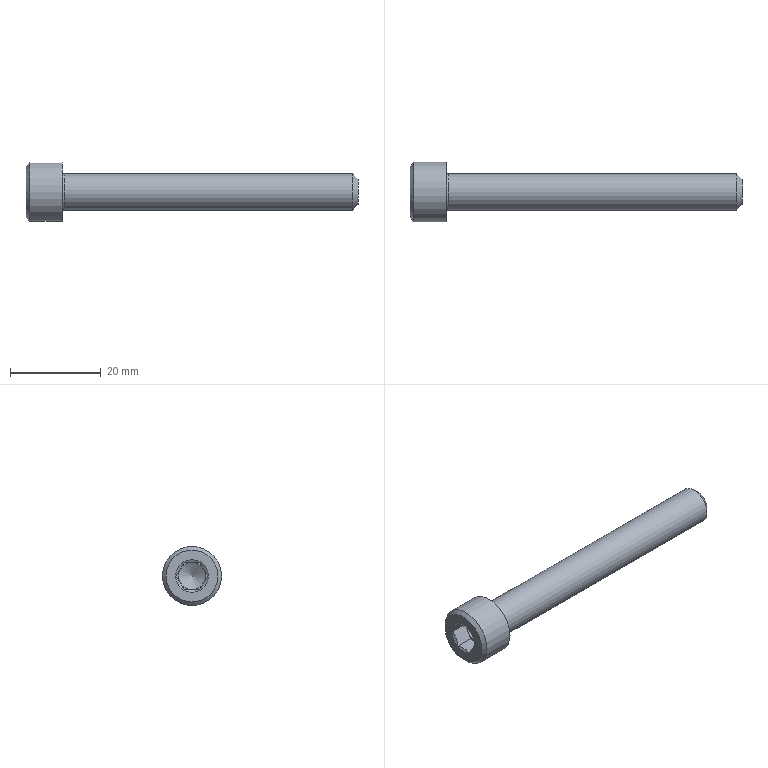Part | STEP file | Винт М8-6gx65 ГОСТ 11738-84 | 1 solid | 23 faces | box 73 x 13 x 13 mm | volume 4129 mm3 | plane 15 | cone 4 | cylinder 3 | torus 1 | commonest cylinder face diameters 6 x1 8 x1 13 x1
STEP:
#1=CARTESIAN_POINT('',(-8.,5.7,0.));
#2=VERTEX_POINT('',#1);
#3=CARTESIAN_POINT('',(-8.,0.,0.));
#4=DIRECTION('',(1.,0.,0.));
#5=DIRECTION('',(0.,1.,0.));
#6=AXIS2_PLACEMENT_3D('',#3,#4,#5);
#7=CIRCLE('',#6,5.7);
#8=EDGE_CURVE('',#2,#2,#7,.T.);
#9=ORIENTED_EDGE('',*,*,#8,.F.);
#10=EDGE_LOOP('',(#9));
#11=FACE_BOUND('',#10,.T.);
#12=CARTESIAN_POINT('',(-8.,3.6,0.));
#13=VERTEX_POINT('',#12);
#14=CARTESIAN_POINT('',(-8.,0.,0.));
#15=DIRECTION('',(1.,0.,0.));
#16=DIRECTION('',(0.,1.,0.));
#17=AXIS2_PLACEMENT_3D('',#14,#15,#16);
#18=CIRCLE('',#17,3.6);
#19=EDGE_CURVE('',#13,#13,#18,.T.);
#20=ORIENTED_EDGE('',*,*,#19,.T.);
#21=EDGE_LOOP('',(#20));
#22=FACE_BOUND('',#21,.T.);
#23=CARTESIAN_POINT('',(-8.,0.,0.));
#24=DIRECTION('',(-1.,0.,0.));
#25=DIRECTION('',(0.,1.,0.));
#26=AXIS2_PLACEMENT_3D('',#23,#24,#25);
#27=PLANE('',#26);
#28=ADVANCED_FACE('',(#11,#22),#27,.T.);
#29=CARTESIAN_POINT('',(-7.922,1.732,-3.));
#30=VERTEX_POINT('',#29);
#31=CARTESIAN_POINT('',(-7.922,-1.732,-3.));
#32=VERTEX_POINT('',#31);
#33=CARTESIAN_POINT('',(-7.922,1.732,-3.));
#34=CARTESIAN_POINT('',(-7.911,1.695,-3.));
#35=CARTESIAN_POINT('',(-7.891,1.625,-3.));
#36=CARTESIAN_POINT('',(-7.871,1.55,-3.));
#37=CARTESIAN_POINT('',(-7.851,1.474,-3.));
#38=CARTESIAN_POINT('',(-7.831,1.391,-3.));
#39=CARTESIAN_POINT('',(-7.803,1.276,-3.));
#40=CARTESIAN_POINT('',(-7.779,1.162,-3.));
#41=CARTESIAN_POINT('',(-7.76,1.068,-3.));
#42=CARTESIAN_POINT('',(-7.736,0.9374,-3.));
#43=CARTESIAN_POINT('',(-7.712,0.7953,-3.));
#44=CARTESIAN_POINT('',(-7.692,0.6398,-3.));
#45=CARTESIAN_POINT('',(-7.676,0.4906,-3.));
#46=CARTESIAN_POINT('',(-7.667,0.3765,-3.));
#47=CARTESIAN_POINT('',(-7.659,0.2523,-3.));
#48=CARTESIAN_POINT('',(-7.655,0.1456,-3.));
#49=CARTESIAN_POINT('',(-7.654,0.04767,-3.));
#50=CARTESIAN_POINT('',(-7.654,-0.05476,-3.));
#51=CARTESIAN_POINT('',(-7.655,-0.115,-3.));
#52=CARTESIAN_POINT('',(-7.658,-0.2282,-3.));
#53=CARTESIAN_POINT('',(-7.665,-0.3516,-3.));
#54=CARTESIAN_POINT('',(-7.676,-0.494,-3.));
#55=CARTESIAN_POINT('',(-7.689,-0.6078,-3.));
#56=CARTESIAN_POINT('',(-7.702,-0.7201,-3.));
#57=CARTESIAN_POINT('',(-7.719,-0.8365,-3.));
#58=CARTESIAN_POINT('',(-7.737,-0.9456,-3.));
#59=CARTESIAN_POINT('',(-7.756,-1.051,-3.));
#60=CARTESIAN_POINT('',(-7.781,-1.173,-3.));
#61=CARTESIAN_POINT('',(-7.808,-1.297,-3.));
#62=CARTESIAN_POINT('',(-7.831,-1.393,-3.));
#63=CARTESIAN_POINT('',(-7.854,-1.486,-3.));
#64=CARTESIAN_POINT('',(-7.882,-1.59,-3.));
#65=CARTESIAN_POINT('',(-7.906,-1.679,-3.));
#66=CARTESIAN_POINT('',(-7.919,-1.723,-3.));
#67=CARTESIAN_POINT('',(-7.922,-1.732,-3.));
#68=B_SPLINE_CURVE_WITH_KNOTS('',3,(#33,#34,#35,#36,#37,#38,#39,#40,#41,#42,#43,#44,#45,#46,#47,#48,#49,#50,#51,#52,#53,#54,#55,#56,#57,#58,#59,#60,#61,#62,#63,#64,#65,#66,#67),.UNSPECIFIED.,.F.,.F.,(4,1,1,1,1,1,1,1,1,1,1,1,1,1,1,1,1,1,1,1,1,1,1,1,1,1,1,1,1,1,1,1,4),(0.,0.03325,0.06137,0.06664,0.1002,0.134,0.1679,0.1994,0.2162,0.2809,0.3222,0.3499,0.4089,0.4198,0.456,0.5,0.5033,0.5434,0.5514,0.5999,0.6487,0.6732,0.6976,0.7453,0.7735,0.7919,0.8363,0.8796,0.9003,0.9208,0.9609,0.9923,1.),.UNSPECIFIED.);
#69=EDGE_CURVE('',#30,#32,#68,.T.);
#70=ORIENTED_EDGE('',*,*,#69,.T.);
#71=CARTESIAN_POINT('',(-4.,-1.732,-3.));
#72=VERTEX_POINT('',#71);
#73=CARTESIAN_POINT('',(-4.,-1.732,-3.));
#74=DIRECTION('',(-1.,0.,0.));
#75=VECTOR('',#74,1.);
#76=LINE('',#73,#75);
#77=EDGE_CURVE('',#72,#32,#76,.T.);
#78=ORIENTED_EDGE('',*,*,#77,.F.);
#79=CARTESIAN_POINT('',(-4.,0.,-3.));
#80=VERTEX_POINT('',#79);
#81=CARTESIAN_POINT('',(-4.,0.,-3.));
#82=DIRECTION('',(0.,-1.,0.));
#83=VECTOR('',#82,1.);
#84=LINE('',#81,#83);
#85=EDGE_CURVE('',#80,#72,#84,.T.);
#86=ORIENTED_EDGE('',*,*,#85,.F.);
#87=CARTESIAN_POINT('',(-4.,1.732,-3.));
#88=VERTEX_POINT('',#87);
#89=CARTESIAN_POINT('',(-4.,1.732,-3.));
#90=DIRECTION('',(0.,-1.,0.));
#91=VECTOR('',#90,1.);
#92=LINE('',#89,#91);
#93=EDGE_CURVE('',#88,#80,#92,.T.);
#94=ORIENTED_EDGE('',*,*,#93,.F.);
#95=CARTESIAN_POINT('',(-4.,1.732,-3.));
#96=DIRECTION('',(-1.,0.,0.));
#97=VECTOR('',#96,1.);
#98=LINE('',#95,#97);
#99=EDGE_CURVE('',#88,#30,#98,.T.);
#100=ORIENTED_EDGE('',*,*,#99,.T.);
#101=EDGE_LOOP('',(#70,#78,#86,#94,#100));
#102=FACE_BOUND('',#101,.T.);
#103=CARTESIAN_POINT('',(-4.,1.732,-3.));
#104=DIRECTION('',(0.,0.,-1.));
#105=DIRECTION('',(0.,-1.,0.));
#106=AXIS2_PLACEMENT_3D('',#103,#104,#105);
#107=PLANE('',#106);
#108=ADVANCED_FACE('',(#102),#107,.F.);
#109=CARTESIAN_POINT('',(-7.922,-3.464,0.));
#110=VERTEX_POINT('',#109);
#111=CARTESIAN_POINT('',(-7.922,-1.732,-3.));
#112=CARTESIAN_POINT('',(-7.911,-1.751,-2.968));
#113=CARTESIAN_POINT('',(-7.89,-1.788,-2.902));
#114=CARTESIAN_POINT('',(-7.859,-1.845,-2.804));
#115=CARTESIAN_POINT('',(-7.831,-1.902,-2.705));
#116=CARTESIAN_POINT('',(-7.803,-1.96,-2.605));
#117=CARTESIAN_POINT('',(-7.775,-2.027,-2.49));
#118=CARTESIAN_POINT('',(-7.741,-2.111,-2.343));
#119=CARTESIAN_POINT('',(-7.707,-2.216,-2.161));
#120=CARTESIAN_POINT('',(-7.68,-2.329,-1.967));
#121=CARTESIAN_POINT('',(-7.663,-2.431,-1.789));
#122=CARTESIAN_POINT('',(-7.655,-2.519,-1.637));
#123=CARTESIAN_POINT('',(-7.654,-2.574,-1.541));
#124=CARTESIAN_POINT('',(-7.654,-2.63,-1.444));
#125=CARTESIAN_POINT('',(-7.656,-2.689,-1.343));
#126=CARTESIAN_POINT('',(-7.665,-2.774,-1.196));
#127=CARTESIAN_POINT('',(-7.679,-2.859,-1.048));
#128=CARTESIAN_POINT('',(-7.698,-2.944,-0.901));
#129=CARTESIAN_POINT('',(-7.722,-3.027,-0.7571));
#130=CARTESIAN_POINT('',(-7.75,-3.107,-0.6183));
#131=CARTESIAN_POINT('',(-7.781,-3.184,-0.4844));
#132=CARTESIAN_POINT('',(-7.813,-3.258,-0.3566));
#133=CARTESIAN_POINT('',(-7.848,-3.329,-0.2336));
#134=CARTESIAN_POINT('',(-7.884,-3.397,-0.1154));
#135=CARTESIAN_POINT('',(-7.909,-3.442,-0.03806));
#136=CARTESIAN_POINT('',(-7.922,-3.464,-0.000000001));
#137=B_SPLINE_CURVE_WITH_KNOTS('',3,(#111,#112,#113,#114,#115,#116,#117,#118,#119,#120,#121,#122,#123,#124,#125,#126,#127,#128,#129,#130,#131,#132,#133,#134,#135,#136),.UNSPECIFIED.,.F.,.F.,(4,1,1,1,1,1,1,1,1,1,1,1,1,1,1,1,1,1,1,1,1,1,1,4),(0.,0.03325,0.06664,0.1002,0.134,0.1679,0.2162,0.2809,0.3499,0.4089,0.456,0.5,0.5033,0.5514,0.5999,0.6487,0.6976,0.7453,0.7919,0.8363,0.8796,0.9208,0.9609,1.),.UNSPECIFIED.);
#138=EDGE_CURVE('',#32,#110,#137,.T.);
#139=ORIENTED_EDGE('',*,*,#138,.T.);
#140=CARTESIAN_POINT('',(-4.,-3.464,0.));
#141=VERTEX_POINT('',#140);
#142=CARTESIAN_POINT('',(-4.,-3.464,0.));
#143=DIRECTION('',(-1.,0.,0.));
#144=VECTOR('',#143,1.);
#145=LINE('',#142,#144);
#146=EDGE_CURVE('',#141,#110,#145,.T.);
#147=ORIENTED_EDGE('',*,*,#146,.F.);
#148=CARTESIAN_POINT('',(-4.,-2.598,-1.5));
#149=VERTEX_POINT('',#148);
#150=CARTESIAN_POINT('',(-4.,-2.598,-1.5));
#151=DIRECTION('',(0.,-0.5,0.866));
#152=VECTOR('',#151,1.);
#153=LINE('',#150,#152);
#154=EDGE_CURVE('',#149,#141,#153,.T.);
#155=ORIENTED_EDGE('',*,*,#154,.F.);
#156=CARTESIAN_POINT('',(-4.,-1.732,-3.));
#157=DIRECTION('',(0.,-0.5,0.866));
#158=VECTOR('',#157,1.);
#159=LINE('',#156,#158);
#160=EDGE_CURVE('',#72,#149,#159,.T.);
#161=ORIENTED_EDGE('',*,*,#160,.F.);
#162=ORIENTED_EDGE('',*,*,#77,.T.);
#163=EDGE_LOOP('',(#139,#147,#155,#161,#162));
#164=FACE_BOUND('',#163,.T.);
#165=CARTESIAN_POINT('',(-4.,-1.732,-3.));
#166=DIRECTION('',(0.,-0.866,-0.5));
#167=DIRECTION('',(0.,-0.5,0.866));
#168=AXIS2_PLACEMENT_3D('',#165,#166,#167);
#169=PLANE('',#168);
#170=ADVANCED_FACE('',(#164),#169,.F.);
#171=CARTESIAN_POINT('',(-7.922,-1.732,3.));
#172=VERTEX_POINT('',#171);
#173=CARTESIAN_POINT('',(-7.922,-3.464,0.));
#174=CARTESIAN_POINT('',(-7.911,-3.445,0.03241));
#175=CARTESIAN_POINT('',(-7.89,-3.408,0.09751));
#176=CARTESIAN_POINT('',(-7.859,-3.351,0.1958));
#177=CARTESIAN_POINT('',(-7.831,-3.294,0.295));
#178=CARTESIAN_POINT('',(-7.803,-3.236,0.3951));
#179=CARTESIAN_POINT('',(-7.775,-3.17,0.5102));
#180=CARTESIAN_POINT('',(-7.741,-3.085,0.6567));
#181=CARTESIAN_POINT('',(-7.707,-2.98,0.839));
#182=CARTESIAN_POINT('',(-7.68,-2.867,1.033));
#183=CARTESIAN_POINT('',(-7.663,-2.765,1.211));
#184=CARTESIAN_POINT('',(-7.655,-2.677,1.363));
#185=CARTESIAN_POINT('',(-7.654,-2.622,1.459));
#186=CARTESIAN_POINT('',(-7.654,-2.566,1.556));
#187=CARTESIAN_POINT('',(-7.656,-2.507,1.657));
#188=CARTESIAN_POINT('',(-7.665,-2.422,1.804));
#189=CARTESIAN_POINT('',(-7.679,-2.337,1.952));
#190=CARTESIAN_POINT('',(-7.698,-2.252,2.099));
#191=CARTESIAN_POINT('',(-7.722,-2.169,2.243));
#192=CARTESIAN_POINT('',(-7.75,-2.089,2.382));
#193=CARTESIAN_POINT('',(-7.781,-2.012,2.516));
#194=CARTESIAN_POINT('',(-7.813,-1.938,2.643));
#195=CARTESIAN_POINT('',(-7.848,-1.867,2.766));
#196=CARTESIAN_POINT('',(-7.884,-1.799,2.885));
#197=CARTESIAN_POINT('',(-7.909,-1.754,2.962));
#198=CARTESIAN_POINT('',(-7.922,-1.732,3.));
#199=B_SPLINE_CURVE_WITH_KNOTS('',3,(#173,#174,#175,#176,#177,#178,#179,#180,#181,#182,#183,#184,#185,#186,#187,#188,#189,#190,#191,#192,#193,#194,#195,#196,#197,#198),.UNSPECIFIED.,.F.,.F.,(4,1,1,1,1,1,1,1,1,1,1,1,1,1,1,1,1,1,1,1,1,1,1,4),(0.,0.03325,0.06664,0.1002,0.134,0.1679,0.2162,0.2809,0.3499,0.4089,0.456,0.5,0.5033,0.5514,0.5999,0.6487,0.6976,0.7453,0.7919,0.8363,0.8796,0.9208,0.9609,1.),.UNSPECIFIED.);
#200=EDGE_CURVE('',#110,#172,#199,.T.);
#201=ORIENTED_EDGE('',*,*,#200,.T.);
#202=CARTESIAN_POINT('',(-4.,-1.732,3.));
#203=VERTEX_POINT('',#202);
#204=CARTESIAN_POINT('',(-4.,-1.732,3.));
#205=DIRECTION('',(-1.,0.,0.));
#206=VECTOR('',#205,1.);
#207=LINE('',#204,#206);
#208=EDGE_CURVE('',#203,#172,#207,.T.);
#209=ORIENTED_EDGE('',*,*,#208,.F.);
#210=CARTESIAN_POINT('',(-4.,-2.598,1.5));
#211=VERTEX_POINT('',#210);
#212=CARTESIAN_POINT('',(-4.,-2.598,1.5));
#213=DIRECTION('',(0.,0.5,0.866));
#214=VECTOR('',#213,1.);
#215=LINE('',#212,#214);
#216=EDGE_CURVE('',#211,#203,#215,.T.);
#217=ORIENTED_EDGE('',*,*,#216,.F.);
#218=CARTESIAN_POINT('',(-4.,-3.464,0.));
#219=DIRECTION('',(0.,0.5,0.866));
#220=VECTOR('',#219,1.);
#221=LINE('',#218,#220);
#222=EDGE_CURVE('',#141,#211,#221,.T.);
#223=ORIENTED_EDGE('',*,*,#222,.F.);
#224=ORIENTED_EDGE('',*,*,#146,.T.);
#225=EDGE_LOOP('',(#201,#209,#217,#223,#224));
#226=FACE_BOUND('',#225,.T.);
#227=CARTESIAN_POINT('',(-4.,-3.464,0.));
#228=DIRECTION('',(0.,-0.866,0.5));
#229=DIRECTION('',(0.,0.5,0.866));
#230=AXIS2_PLACEMENT_3D('',#227,#228,#229);
#231=PLANE('',#230);
#232=ADVANCED_FACE('',(#226),#231,.F.);
#233=CARTESIAN_POINT('',(-7.922,1.732,3.));
#234=VERTEX_POINT('',#233);
#235=CARTESIAN_POINT('',(-7.922,-1.732,3.));
#236=CARTESIAN_POINT('',(-7.911,-1.695,3.));
#237=CARTESIAN_POINT('',(-7.891,-1.625,3.));
#238=CARTESIAN_POINT('',(-7.871,-1.55,3.));
#239=CARTESIAN_POINT('',(-7.851,-1.474,3.));
#240=CARTESIAN_POINT('',(-7.831,-1.391,3.));
#241=CARTESIAN_POINT('',(-7.803,-1.276,3.));
#242=CARTESIAN_POINT('',(-7.779,-1.162,3.));
#243=CARTESIAN_POINT('',(-7.76,-1.068,3.));
#244=CARTESIAN_POINT('',(-7.736,-0.9374,3.));
#245=CARTESIAN_POINT('',(-7.712,-0.7953,3.));
#246=CARTESIAN_POINT('',(-7.692,-0.6398,3.));
#247=CARTESIAN_POINT('',(-7.676,-0.4906,3.));
#248=CARTESIAN_POINT('',(-7.667,-0.3765,3.));
#249=CARTESIAN_POINT('',(-7.659,-0.2523,3.));
#250=CARTESIAN_POINT('',(-7.655,-0.1456,3.));
#251=CARTESIAN_POINT('',(-7.654,-0.04767,3.));
#252=CARTESIAN_POINT('',(-7.654,0.05476,3.));
#253=CARTESIAN_POINT('',(-7.655,0.115,3.));
#254=CARTESIAN_POINT('',(-7.658,0.2282,3.));
#255=CARTESIAN_POINT('',(-7.665,0.3516,3.));
#256=CARTESIAN_POINT('',(-7.676,0.494,3.));
#257=CARTESIAN_POINT('',(-7.689,0.6078,3.));
#258=CARTESIAN_POINT('',(-7.702,0.7201,3.));
#259=CARTESIAN_POINT('',(-7.719,0.8365,3.));
#260=CARTESIAN_POINT('',(-7.737,0.9456,3.));
#261=CARTESIAN_POINT('',(-7.756,1.051,3.));
#262=CARTESIAN_POINT('',(-7.781,1.173,3.));
#263=CARTESIAN_POINT('',(-7.808,1.297,3.));
#264=CARTESIAN_POINT('',(-7.831,1.393,3.));
#265=CARTESIAN_POINT('',(-7.854,1.486,3.));
#266=CARTESIAN_POINT('',(-7.882,1.59,3.));
#267=CARTESIAN_POINT('',(-7.906,1.679,3.));
#268=CARTESIAN_POINT('',(-7.919,1.723,3.));
#269=CARTESIAN_POINT('',(-7.922,1.732,3.));
#270=B_SPLINE_CURVE_WITH_KNOTS('',3,(#235,#236,#237,#238,#239,#240,#241,#242,#243,#244,#245,#246,#247,#248,#249,#250,#251,#252,#253,#254,#255,#256,#257,#258,#259,#260,#261,#262,#263,#264,#265,#266,#267,#268,#269),.UNSPECIFIED.,.F.,.F.,(4,1,1,1,1,1,1,1,1,1,1,1,1,1,1,1,1,1,1,1,1,1,1,1,1,1,1,1,1,1,1,1,4),(0.,0.03325,0.06137,0.06664,0.1002,0.134,0.1679,0.1994,0.2162,0.2809,0.3222,0.3499,0.4089,0.4198,0.456,0.5,0.5033,0.5434,0.5514,0.5999,0.6487,0.6732,0.6976,0.7453,0.7735,0.7919,0.8363,0.8796,0.9003,0.9208,0.9609,0.9923,1.),.UNSPECIFIED.);
#271=EDGE_CURVE('',#172,#234,#270,.T.);
#272=ORIENTED_EDGE('',*,*,#271,.T.);
#273=CARTESIAN_POINT('',(-4.,1.732,3.));
#274=VERTEX_POINT('',#273);
#275=CARTESIAN_POINT('',(-4.,1.732,3.));
#276=DIRECTION('',(-1.,0.,0.));
#277=VECTOR('',#276,1.);
#278=LINE('',#275,#277);
#279=EDGE_CURVE('',#274,#234,#278,.T.);
#280=ORIENTED_EDGE('',*,*,#279,.F.);
#281=CARTESIAN_POINT('',(-4.,0.,3.));
#282=VERTEX_POINT('',#281);
#283=CARTESIAN_POINT('',(-4.,0.,3.));
#284=DIRECTION('',(0.,1.,0.));
#285=VECTOR('',#284,1.);
#286=LINE('',#283,#285);
#287=EDGE_CURVE('',#282,#274,#286,.T.);
#288=ORIENTED_EDGE('',*,*,#287,.F.);
#289=CARTESIAN_POINT('',(-4.,-1.732,3.));
#290=DIRECTION('',(0.,1.,0.));
#291=VECTOR('',#290,1.);
#292=LINE('',#289,#291);
#293=EDGE_CURVE('',#203,#282,#292,.T.);
#294=ORIENTED_EDGE('',*,*,#293,.F.);
#295=ORIENTED_EDGE('',*,*,#208,.T.);
#296=EDGE_LOOP('',(#272,#280,#288,#294,#295));
#297=FACE_BOUND('',#296,.T.);
#298=CARTESIAN_POINT('',(-4.,-1.732,3.));
#299=DIRECTION('',(0.,0.,1.));
#300=DIRECTION('',(0.,1.,0.));
#301=AXIS2_PLACEMENT_3D('',#298,#299,#300);
#302=PLANE('',#301);
#303=ADVANCED_FACE('',(#297),#302,.F.);
#304=CARTESIAN_POINT('',(-7.922,3.464,0.));
#305=VERTEX_POINT('',#304);
#306=CARTESIAN_POINT('',(-7.922,3.464,0.));
#307=CARTESIAN_POINT('',(-7.911,3.445,-0.03242));
#308=CARTESIAN_POINT('',(-7.89,3.408,-0.09751));
#309=CARTESIAN_POINT('',(-7.859,3.351,-0.1958));
#310=CARTESIAN_POINT('',(-7.831,3.294,-0.295));
#311=CARTESIAN_POINT('',(-7.803,3.236,-0.3951));
#312=CARTESIAN_POINT('',(-7.775,3.17,-0.5102));
#313=CARTESIAN_POINT('',(-7.741,3.085,-0.6567));
#314=CARTESIAN_POINT('',(-7.707,2.98,-0.839));
#315=CARTESIAN_POINT('',(-7.68,2.867,-1.033));
#316=CARTESIAN_POINT('',(-7.663,2.765,-1.211));
#317=CARTESIAN_POINT('',(-7.655,2.677,-1.363));
#318=CARTESIAN_POINT('',(-7.654,2.622,-1.459));
#319=CARTESIAN_POINT('',(-7.654,2.566,-1.556));
#320=CARTESIAN_POINT('',(-7.656,2.507,-1.657));
#321=CARTESIAN_POINT('',(-7.665,2.422,-1.805));
#322=CARTESIAN_POINT('',(-7.679,2.337,-1.952));
#323=CARTESIAN_POINT('',(-7.698,2.252,-2.099));
#324=CARTESIAN_POINT('',(-7.722,2.169,-2.243));
#325=CARTESIAN_POINT('',(-7.75,2.089,-2.382));
#326=CARTESIAN_POINT('',(-7.781,2.012,-2.516));
#327=CARTESIAN_POINT('',(-7.813,1.938,-2.643));
#328=CARTESIAN_POINT('',(-7.848,1.867,-2.766));
#329=CARTESIAN_POINT('',(-7.884,1.799,-2.885));
#330=CARTESIAN_POINT('',(-7.909,1.754,-2.962));
#331=CARTESIAN_POINT('',(-7.922,1.732,-3.));
#332=B_SPLINE_CURVE_WITH_KNOTS('',3,(#306,#307,#308,#309,#310,#311,#312,#313,#314,#315,#316,#317,#318,#319,#320,#321,#322,#323,#324,#325,#326,#327,#328,#329,#330,#331),.UNSPECIFIED.,.F.,.F.,(4,1,1,1,1,1,1,1,1,1,1,1,1,1,1,1,1,1,1,1,1,1,1,4),(0.,0.03325,0.06664,0.1002,0.134,0.1679,0.2162,0.2809,0.3499,0.4089,0.456,0.5,0.5033,0.5514,0.5999,0.6487,0.6976,0.7453,0.7919,0.8363,0.8796,0.9208,0.9609,1.),.UNSPECIFIED.);
#333=EDGE_CURVE('',#305,#30,#332,.T.);
#334=ORIENTED_EDGE('',*,*,#333,.T.);
#335=ORIENTED_EDGE('',*,*,#99,.F.);
#336=CARTESIAN_POINT('',(-4.,2.598,-1.5));
#337=VERTEX_POINT('',#336);
#338=CARTESIAN_POINT('',(-4.,2.598,-1.5));
#339=DIRECTION('',(0.,-0.5,-0.866));
#340=VECTOR('',#339,1.);
#341=LINE('',#338,#340);
#342=EDGE_CURVE('',#337,#88,#341,.T.);
#343=ORIENTED_EDGE('',*,*,#342,.F.);
#344=CARTESIAN_POINT('',(-4.,3.464,0.));
#345=VERTEX_POINT('',#344);
#346=CARTESIAN_POINT('',(-4.,3.464,0.));
#347=DIRECTION('',(0.,-0.5,-0.866));
#348=VECTOR('',#347,1.);
#349=LINE('',#346,#348);
#350=EDGE_CURVE('',#345,#337,#349,.T.);
#351=ORIENTED_EDGE('',*,*,#350,.F.);
#352=CARTESIAN_POINT('',(-4.,3.464,0.));
#353=DIRECTION('',(-1.,0.,0.));
#354=VECTOR('',#353,1.);
#355=LINE('',#352,#354);
#356=EDGE_CURVE('',#345,#305,#355,.T.);
#357=ORIENTED_EDGE('',*,*,#356,.T.);
#358=EDGE_LOOP('',(#334,#335,#343,#351,#357));
#359=FACE_BOUND('',#358,.T.);
#360=CARTESIAN_POINT('',(-4.,3.464,0.));
#361=DIRECTION('',(0.,0.866,-0.5));
#362=DIRECTION('',(0.,-0.5,-0.866));
#363=AXIS2_PLACEMENT_3D('',#360,#361,#362);
#364=PLANE('',#363);
#365=ADVANCED_FACE('',(#359),#364,.F.);
#366=CARTESIAN_POINT('',(-7.922,1.732,3.));
#367=CARTESIAN_POINT('',(-7.911,1.751,2.968));
#368=CARTESIAN_POINT('',(-7.89,1.788,2.902));
#369=CARTESIAN_POINT('',(-7.859,1.845,2.804));
#370=CARTESIAN_POINT('',(-7.831,1.902,2.705));
#371=CARTESIAN_POINT('',(-7.803,1.96,2.605));
#372=CARTESIAN_POINT('',(-7.775,2.027,2.49));
#373=CARTESIAN_POINT('',(-7.741,2.111,2.343));
#374=CARTESIAN_POINT('',(-7.707,2.216,2.161));
#375=CARTESIAN_POINT('',(-7.68,2.329,1.967));
#376=CARTESIAN_POINT('',(-7.663,2.431,1.789));
#377=CARTESIAN_POINT('',(-7.655,2.519,1.637));
#378=CARTESIAN_POINT('',(-7.654,2.574,1.541));
#379=CARTESIAN_POINT('',(-7.654,2.63,1.444));
#380=CARTESIAN_POINT('',(-7.656,2.689,1.343));
#381=CARTESIAN_POINT('',(-7.665,2.774,1.195));
#382=CARTESIAN_POINT('',(-7.679,2.859,1.048));
#383=CARTESIAN_POINT('',(-7.698,2.944,0.9009));
#384=CARTESIAN_POINT('',(-7.722,3.027,0.7571));
#385=CARTESIAN_POINT('',(-7.75,3.107,0.6183));
#386=CARTESIAN_POINT('',(-7.781,3.184,0.4844));
#387=CARTESIAN_POINT('',(-7.813,3.258,0.3566));
#388=CARTESIAN_POINT('',(-7.848,3.329,0.2336));
#389=CARTESIAN_POINT('',(-7.884,3.397,0.1154));
#390=CARTESIAN_POINT('',(-7.909,3.442,0.03806));
#391=CARTESIAN_POINT('',(-7.922,3.464,0.));
#392=B_SPLINE_CURVE_WITH_KNOTS('',3,(#366,#367,#368,#369,#370,#371,#372,#373,#374,#375,#376,#377,#378,#379,#380,#381,#382,#383,#384,#385,#386,#387,#388,#389,#390,#391),.UNSPECIFIED.,.F.,.F.,(4,1,1,1,1,1,1,1,1,1,1,1,1,1,1,1,1,1,1,1,1,1,1,4),(0.,0.03325,0.06664,0.1002,0.134,0.1679,0.2162,0.2809,0.3499,0.4089,0.456,0.5,0.5033,0.5514,0.5999,0.6487,0.6976,0.7453,0.7919,0.8363,0.8796,0.9208,0.9609,1.),.UNSPECIFIED.);
#393=EDGE_CURVE('',#234,#305,#392,.T.);
#394=ORIENTED_EDGE('',*,*,#393,.T.);
#395=ORIENTED_EDGE('',*,*,#356,.F.);
#396=CARTESIAN_POINT('',(-4.,2.598,1.5));
#397=VERTEX_POINT('',#396);
#398=CARTESIAN_POINT('',(-4.,2.598,1.5));
#399=DIRECTION('',(0.,0.5,-0.866));
#400=VECTOR('',#399,1.);
#401=LINE('',#398,#400);
#402=EDGE_CURVE('',#397,#345,#401,.T.);
#403=ORIENTED_EDGE('',*,*,#402,.F.);
#404=CARTESIAN_POINT('',(-4.,1.732,3.));
#405=DIRECTION('',(0.,0.5,-0.866));
#406=VECTOR('',#405,1.);
#407=LINE('',#404,#406);
#408=EDGE_CURVE('',#274,#397,#407,.T.);
#409=ORIENTED_EDGE('',*,*,#408,.F.);
#410=ORIENTED_EDGE('',*,*,#279,.T.);
#411=EDGE_LOOP('',(#394,#395,#403,#409,#410));
#412=FACE_BOUND('',#411,.T.);
#413=CARTESIAN_POINT('',(-4.,1.732,3.));
#414=DIRECTION('',(0.,0.866,0.5));
#415=DIRECTION('',(0.,0.5,-0.866));
#416=AXIS2_PLACEMENT_3D('',#413,#414,#415);
#417=PLANE('',#416);
#418=ADVANCED_FACE('',(#412),#417,.F.);
#419=ORIENTED_EDGE('',*,*,#393,.F.);
#420=ORIENTED_EDGE('',*,*,#271,.F.);
#421=ORIENTED_EDGE('',*,*,#200,.F.);
#422=ORIENTED_EDGE('',*,*,#138,.F.);
#423=ORIENTED_EDGE('',*,*,#69,.F.);
#424=ORIENTED_EDGE('',*,*,#333,.F.);
#425=EDGE_LOOP('',(#419,#420,#421,#422,#423,#424));
#426=FACE_BOUND('',#425,.T.);
#427=ORIENTED_EDGE('',*,*,#19,.F.);
#428=EDGE_LOOP('',(#427));
#429=FACE_OUTER_BOUND('',#428,.T.);
#430=CARTESIAN_POINT('',(-7.827,0.,0.));
#431=DIRECTION('',(-1.,0.,0.));
#432=DIRECTION('',(0.,-1.,0.));
#433=AXIS2_PLACEMENT_3D('',#430,#431,#432);
#434=CONICAL_SURFACE('',#433,3.3,1.047);
#435=ADVANCED_FACE('',(#426,#429),#434,.F.);
#436=CARTESIAN_POINT('',(-7.2,6.5,0.));
#437=VERTEX_POINT('',#436);
#438=CARTESIAN_POINT('',(-7.2,0.,0.));
#439=DIRECTION('',(1.,0.,0.));
#440=DIRECTION('',(0.,1.,0.));
#441=AXIS2_PLACEMENT_3D('',#438,#439,#440);
#442=CIRCLE('',#441,6.5);
#443=EDGE_CURVE('',#437,#437,#442,.T.);
#444=ORIENTED_EDGE('',*,*,#443,.F.);
#445=EDGE_LOOP('',(#444));
#446=FACE_OUTER_BOUND('',#445,.T.);
#447=ORIENTED_EDGE('',*,*,#8,.T.);
#448=EDGE_LOOP('',(#447));
#449=FACE_OUTER_BOUND('',#448,.T.);
#450=CARTESIAN_POINT('',(-7.6,0.,0.));
#451=DIRECTION('',(1.,0.,0.));
#452=DIRECTION('',(0.,1.,0.));
#453=AXIS2_PLACEMENT_3D('',#450,#451,#452);
#454=CONICAL_SURFACE('',#453,6.1,0.7854);
#455=ADVANCED_FACE('',(#446,#449),#454,.T.);
#456=CARTESIAN_POINT('',(-4.,0.,0.));
#457=DIRECTION('',(1.,0.,0.));
#458=DIRECTION('',(0.,-0.866,-0.5));
#459=AXIS2_PLACEMENT_3D('',#456,#457,#458);
#460=CIRCLE('',#459,3.);
#461=EDGE_CURVE('',#149,#80,#460,.T.);
#462=ORIENTED_EDGE('',*,*,#461,.T.);
#463=ORIENTED_EDGE('',*,*,#85,.T.);
#464=ORIENTED_EDGE('',*,*,#160,.T.);
#465=EDGE_LOOP('',(#462,#463,#464));
#466=FACE_BOUND('',#465,.T.);
#467=CARTESIAN_POINT('',(-4.,0.,0.));
#468=DIRECTION('',(-1.,0.,0.));
#469=DIRECTION('',(0.,0.,-1.));
#470=AXIS2_PLACEMENT_3D('',#467,#468,#469);
#471=PLANE('',#470);
#472=ADVANCED_FACE('',(#466),#471,.T.);
#473=CARTESIAN_POINT('',(-4.,0.,0.));
#474=DIRECTION('',(1.,0.,0.));
#475=DIRECTION('',(0.,0.,-1.));
#476=AXIS2_PLACEMENT_3D('',#473,#474,#475);
#477=CIRCLE('',#476,3.);
#478=EDGE_CURVE('',#80,#337,#477,.T.);
#479=ORIENTED_EDGE('',*,*,#478,.T.);
#480=ORIENTED_EDGE('',*,*,#342,.T.);
#481=ORIENTED_EDGE('',*,*,#93,.T.);
#482=EDGE_LOOP('',(#479,#480,#481));
#483=FACE_BOUND('',#482,.T.);
#484=CARTESIAN_POINT('',(-4.,0.,0.));
#485=DIRECTION('',(-1.,0.,0.));
#486=DIRECTION('',(0.,0.,-1.));
#487=AXIS2_PLACEMENT_3D('',#484,#485,#486);
#488=PLANE('',#487);
#489=ADVANCED_FACE('',(#483),#488,.T.);
#490=CARTESIAN_POINT('',(-4.,0.,0.));
#491=DIRECTION('',(1.,0.,0.));
#492=DIRECTION('',(0.,-0.866,0.5));
#493=AXIS2_PLACEMENT_3D('',#490,#491,#492);
#494=CIRCLE('',#493,3.);
#495=EDGE_CURVE('',#211,#149,#494,.T.);
#496=ORIENTED_EDGE('',*,*,#495,.T.);
#497=ORIENTED_EDGE('',*,*,#154,.T.);
#498=ORIENTED_EDGE('',*,*,#222,.T.);
#499=EDGE_LOOP('',(#496,#497,#498));
#500=FACE_BOUND('',#499,.T.);
#501=CARTESIAN_POINT('',(-4.,0.,0.));
#502=DIRECTION('',(-1.,0.,0.));
#503=DIRECTION('',(0.,0.,-1.));
#504=AXIS2_PLACEMENT_3D('',#501,#502,#503);
#505=PLANE('',#504);
#506=ADVANCED_FACE('',(#500),#505,.T.);
#507=CARTESIAN_POINT('',(-4.,0.,0.));
#508=DIRECTION('',(1.,0.,0.));
#509=DIRECTION('',(0.,0.,1.));
#510=AXIS2_PLACEMENT_3D('',#507,#508,#509);
#511=CIRCLE('',#510,3.);
#512=EDGE_CURVE('',#282,#211,#511,.T.);
#513=ORIENTED_EDGE('',*,*,#512,.T.);
#514=ORIENTED_EDGE('',*,*,#216,.T.);
#515=ORIENTED_EDGE('',*,*,#293,.T.);
#516=EDGE_LOOP('',(#513,#514,#515));
#517=FACE_BOUND('',#516,.T.);
#518=CARTESIAN_POINT('',(-4.,0.,0.));
#519=DIRECTION('',(-1.,0.,0.));
#520=DIRECTION('',(0.,0.,-1.));
#521=AXIS2_PLACEMENT_3D('',#518,#519,#520);
#522=PLANE('',#521);
#523=ADVANCED_FACE('',(#517),#522,.T.);
#524=CARTESIAN_POINT('',(-4.,0.,0.));
#525=DIRECTION('',(1.,0.,0.));
#526=DIRECTION('',(0.,0.866,0.5));
#527=AXIS2_PLACEMENT_3D('',#524,#525,#526);
#528=CIRCLE('',#527,3.);
#529=EDGE_CURVE('',#397,#282,#528,.T.);
#530=ORIENTED_EDGE('',*,*,#529,.T.);
#531=ORIENTED_EDGE('',*,*,#287,.T.);
#532=ORIENTED_EDGE('',*,*,#408,.T.);
#533=EDGE_LOOP('',(#530,#531,#532));
#534=FACE_BOUND('',#533,.T.);
#535=CARTESIAN_POINT('',(-4.,0.,0.));
#536=DIRECTION('',(-1.,0.,0.));
#537=DIRECTION('',(0.,0.,-1.));
#538=AXIS2_PLACEMENT_3D('',#535,#536,#537);
#539=PLANE('',#538);
#540=ADVANCED_FACE('',(#534),#539,.T.);
#541=CARTESIAN_POINT('',(-4.,3.,0.));
#542=VERTEX_POINT('',#541);
#543=CARTESIAN_POINT('',(-4.,0.,0.));
#544=DIRECTION('',(1.,0.,0.));
#545=DIRECTION('',(0.,1.,0.));
#546=AXIS2_PLACEMENT_3D('',#543,#544,#545);
#547=CIRCLE('',#546,3.);
#548=EDGE_CURVE('',#542,#397,#547,.T.);
#549=ORIENTED_EDGE('',*,*,#548,.T.);
#550=ORIENTED_EDGE('',*,*,#402,.T.);
#551=ORIENTED_EDGE('',*,*,#350,.T.);
#552=CARTESIAN_POINT('',(-4.,0.,0.));
#553=DIRECTION('',(1.,0.,0.));
#554=DIRECTION('',(0.,0.866,-0.5));
#555=AXIS2_PLACEMENT_3D('',#552,#553,#554);
#556=CIRCLE('',#555,3.);
#557=EDGE_CURVE('',#337,#542,#556,.T.);
#558=ORIENTED_EDGE('',*,*,#557,.T.);
#559=EDGE_LOOP('',(#549,#550,#551,#558));
#560=FACE_BOUND('',#559,.T.);
#561=CARTESIAN_POINT('',(-4.,0.,0.));
#562=DIRECTION('',(-1.,0.,0.));
#563=DIRECTION('',(0.,0.,-1.));
#564=AXIS2_PLACEMENT_3D('',#561,#562,#563);
#565=PLANE('',#564);
#566=ADVANCED_FACE('',(#560),#565,.T.);
#567=CARTESIAN_POINT('',(0.,6.5,0.));
#568=VERTEX_POINT('',#567);
#569=CARTESIAN_POINT('',(0.,0.,0.));
#570=DIRECTION('',(1.,0.,0.));
#571=DIRECTION('',(0.,1.,0.));
#572=AXIS2_PLACEMENT_3D('',#569,#570,#571);
#573=CIRCLE('',#572,6.5);
#574=EDGE_CURVE('',#568,#568,#573,.T.);
#575=ORIENTED_EDGE('',*,*,#574,.F.);
#576=EDGE_LOOP('',(#575));
#577=FACE_OUTER_BOUND('',#576,.T.);
#578=ORIENTED_EDGE('',*,*,#443,.T.);
#579=EDGE_LOOP('',(#578));
#580=FACE_OUTER_BOUND('',#579,.T.);
#581=CARTESIAN_POINT('',(-8.,0.,0.));
#582=DIRECTION('',(1.,0.,0.));
#583=DIRECTION('',(0.,1.,0.));
#584=AXIS2_PLACEMENT_3D('',#581,#582,#583);
#585=CYLINDRICAL_SURFACE('',#584,6.5);
#586=ADVANCED_FACE('',(#577,#580),#585,.T.);
#587=CARTESIAN_POINT('',(-3.,3.,0.));
#588=VERTEX_POINT('',#587);
#589=CARTESIAN_POINT('',(-3.,0.,0.));
#590=DIRECTION('',(1.,0.,0.));
#591=DIRECTION('',(0.,1.,0.));
#592=AXIS2_PLACEMENT_3D('',#589,#590,#591);
#593=CIRCLE('',#592,3.);
#594=EDGE_CURVE('',#588,#588,#593,.T.);
#595=ORIENTED_EDGE('',*,*,#594,.T.);
#596=EDGE_LOOP('',(#595));
#597=FACE_OUTER_BOUND('',#596,.T.);
#598=ORIENTED_EDGE('',*,*,#557,.F.);
#599=ORIENTED_EDGE('',*,*,#478,.F.);
#600=ORIENTED_EDGE('',*,*,#461,.F.);
#601=ORIENTED_EDGE('',*,*,#495,.F.);
#602=ORIENTED_EDGE('',*,*,#512,.F.);
#603=ORIENTED_EDGE('',*,*,#529,.F.);
#604=ORIENTED_EDGE('',*,*,#548,.F.);
#605=EDGE_LOOP('',(#598,#599,#600,#601,#602,#603,#604));
#606=FACE_BOUND('',#605,.T.);
#607=CARTESIAN_POINT('',(-8.,0.,0.));
#608=DIRECTION('',(1.,0.,0.));
#609=DIRECTION('',(0.,1.,0.));
#610=AXIS2_PLACEMENT_3D('',#607,#608,#609);
#611=CYLINDRICAL_SURFACE('',#610,3.);
#612=ADVANCED_FACE('',(#597,#606),#611,.F.);
#613=ORIENTED_EDGE('',*,*,#574,.T.);
#614=EDGE_LOOP('',(#613));
#615=FACE_BOUND('',#614,.T.);
#616=CARTESIAN_POINT('',(0.,0.,-4.4));
#617=VERTEX_POINT('',#616);
#618=CARTESIAN_POINT('',(0.,0.,0.));
#619=DIRECTION('',(-1.,0.,0.));
#620=DIRECTION('',(0.,0.,-1.));
#621=AXIS2_PLACEMENT_3D('',#618,#619,#620);
#622=CIRCLE('',#621,4.4);
#623=EDGE_CURVE('',#617,#617,#622,.T.);
#624=ORIENTED_EDGE('',*,*,#623,.T.);
#625=EDGE_LOOP('',(#624));
#626=FACE_BOUND('',#625,.T.);
#627=CARTESIAN_POINT('',(0.,0.,0.));
#628=DIRECTION('',(1.,0.,0.));
#629=DIRECTION('',(0.,1.,0.));
#630=AXIS2_PLACEMENT_3D('',#627,#628,#629);
#631=PLANE('',#630);
#632=ADVANCED_FACE('',(#615,#626),#631,.T.);
#633=ORIENTED_EDGE('',*,*,#594,.F.);
#634=EDGE_LOOP('',(#633));
#635=FACE_OUTER_BOUND('',#634,.T.);
#636=CARTESIAN_POINT('',(-2.134,0.,0.));
#637=DIRECTION('',(-1.,0.,0.));
#638=DIRECTION('',(0.,-1.,0.));
#639=AXIS2_PLACEMENT_3D('',#636,#637,#638);
#640=CONICAL_SURFACE('',#639,1.5,1.047);
#641=ADVANCED_FACE('',(#635),#640,.F.);
#642=CARTESIAN_POINT('',(0.4,0.,-4.));
#643=VERTEX_POINT('',#642);
#644=CARTESIAN_POINT('',(0.4,0.,0.));
#645=DIRECTION('',(-1.,0.,0.));
#646=DIRECTION('',(0.,0.,-1.));
#647=AXIS2_PLACEMENT_3D('',#644,#645,#646);
#648=CIRCLE('',#647,4.);
#649=EDGE_CURVE('',#643,#643,#648,.T.);
#650=ORIENTED_EDGE('',*,*,#649,.T.);
#651=EDGE_LOOP('',(#650));
#652=FACE_OUTER_BOUND('',#651,.T.);
#653=ORIENTED_EDGE('',*,*,#623,.F.);
#654=EDGE_LOOP('',(#653));
#655=FACE_OUTER_BOUND('',#654,.T.);
#656=CARTESIAN_POINT('',(0.4,0.,0.));
#657=DIRECTION('',(-1.,0.,0.));
#658=DIRECTION('',(0.,0.,-1.));
#659=AXIS2_PLACEMENT_3D('',#656,#657,#658);
#660=TOROIDAL_SURFACE('',#659,4.4,0.4);
#661=ADVANCED_FACE('',(#652,#655),#660,.F.);
#662=CARTESIAN_POINT('',(63.75,0.,-4.));
#663=VERTEX_POINT('',#662);
#664=CARTESIAN_POINT('',(63.75,0.,0.));
#665=DIRECTION('',(-1.,0.,0.));
#666=DIRECTION('',(0.,0.,-1.));
#667=AXIS2_PLACEMENT_3D('',#664,#665,#666);
#668=CIRCLE('',#667,4.);
#669=EDGE_CURVE('',#663,#663,#668,.T.);
#670=ORIENTED_EDGE('',*,*,#669,.T.);
#671=EDGE_LOOP('',(#670));
#672=FACE_OUTER_BOUND('',#671,.T.);
#673=ORIENTED_EDGE('',*,*,#649,.F.);
#674=EDGE_LOOP('',(#673));
#675=FACE_OUTER_BOUND('',#674,.T.);
#676=CARTESIAN_POINT('',(65.,0.,0.));
#677=DIRECTION('',(-1.,0.,0.));
#678=DIRECTION('',(0.,0.,-1.));
#679=AXIS2_PLACEMENT_3D('',#676,#677,#678);
#680=CYLINDRICAL_SURFACE('',#679,4.);
#681=ADVANCED_FACE('',(#672,#675),#680,.T.);
#682=CARTESIAN_POINT('',(65.,0.,-2.75));
#683=VERTEX_POINT('',#682);
#684=CARTESIAN_POINT('',(65.,0.,0.));
#685=DIRECTION('',(-1.,0.,0.));
#686=DIRECTION('',(0.,0.,-1.));
#687=AXIS2_PLACEMENT_3D('',#684,#685,#686);
#688=CIRCLE('',#687,2.75);
#689=EDGE_CURVE('',#683,#683,#688,.T.);
#690=ORIENTED_EDGE('',*,*,#689,.F.);
#691=EDGE_LOOP('',(#690));
#692=FACE_BOUND('',#691,.T.);
#693=CARTESIAN_POINT('',(65.,0.,0.));
#694=DIRECTION('',(-1.,0.,0.));
#695=DIRECTION('',(0.,0.,-1.));
#696=AXIS2_PLACEMENT_3D('',#693,#694,#695);
#697=PLANE('',#696);
#698=ADVANCED_FACE('',(#692),#697,.F.);
#699=ORIENTED_EDGE('',*,*,#689,.T.);
#700=EDGE_LOOP('',(#699));
#701=FACE_OUTER_BOUND('',#700,.T.);
#702=ORIENTED_EDGE('',*,*,#669,.F.);
#703=EDGE_LOOP('',(#702));
#704=FACE_OUTER_BOUND('',#703,.T.);
#705=CARTESIAN_POINT('',(64.375,0.,0.));
#706=DIRECTION('',(-1.,0.,0.));
#707=DIRECTION('',(0.,0.,-1.));
#708=AXIS2_PLACEMENT_3D('',#705,#706,#707);
#709=CONICAL_SURFACE('',#708,3.375,0.7854);
#710=ADVANCED_FACE('',(#701,#704),#709,.T.);
#711=CLOSED_SHELL('',(#28,#108,#170,#232,#303,#365,#418,#435,#455,#472,#489,#506,#523,#540,#566,#586,#612,#632,#641,#661,#681,#698,#710));
#712=MANIFOLD_SOLID_BREP('',#711);
#713=(LENGTH_UNIT()NAMED_UNIT(*)SI_UNIT(.MILLI.,.METRE.));
#714=UNCERTAINTY_MEASURE_WITH_UNIT(LENGTH_MEASURE(0.00001),#713,'','');
#715=(NAMED_UNIT(*)PLANE_ANGLE_UNIT()SI_UNIT($,.RADIAN.));
#716=(NAMED_UNIT(*)SI_UNIT($,.STERADIAN.)SOLID_ANGLE_UNIT());
#717=(GEOMETRIC_REPRESENTATION_CONTEXT(3)GLOBAL_UNCERTAINTY_ASSIGNED_CONTEXT((#714))GLOBAL_UNIT_ASSIGNED_CONTEXT((#713,#715,#716))REPRESENTATION_CONTEXT('',''));
#718=ADVANCED_BREP_SHAPE_REPRESENTATION('',(#712),#717);